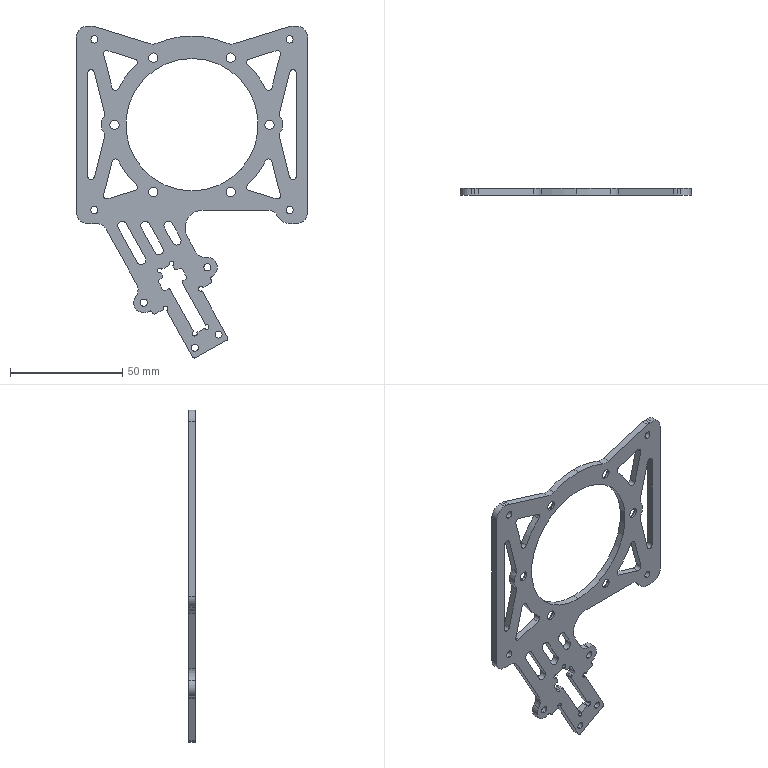Part | SolidWorks | features Fillet 3, Extrusion 1, HoleWzd 1, ICE 1 | 1 solid | 187 faces | box 103 x 3 x 147.909 mm | volume 16759 mm3 | cylinder 121 | plane 54 | cone 12 | commonest cylinder face diameters 3 x24 2 x19 2.1 x13 10 x13 3.2 x12 4.2 x12